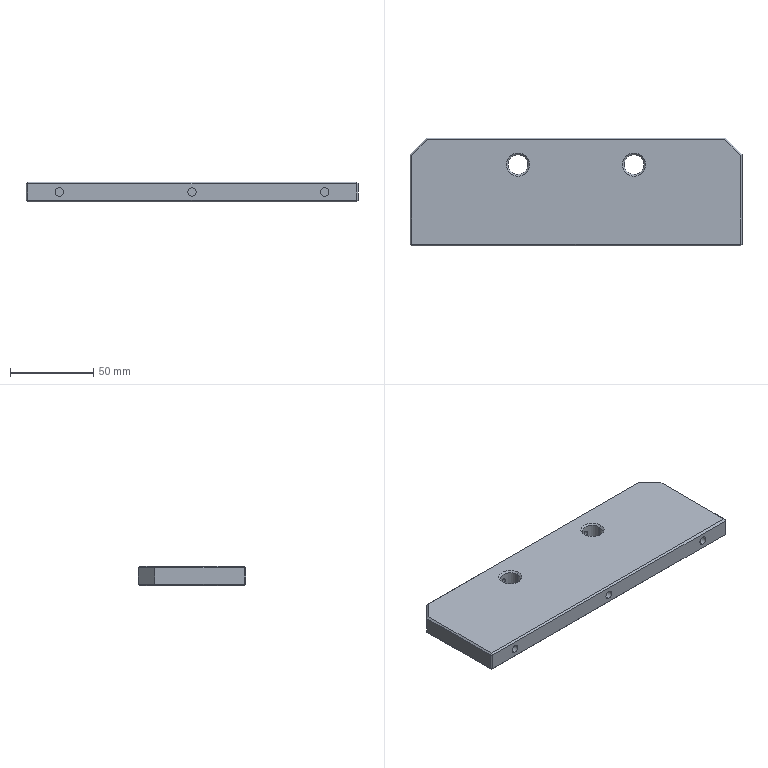Part | STEP file | Rotor mismatch side plate | 1 solid | 51 faces | box 200 x 65 x 12 mm | volume 150424 mm3 | plane 29 | cylinder 14 | cone 8 | commonest cylinder face diameters 5 x6 3.3 x4 12 x4